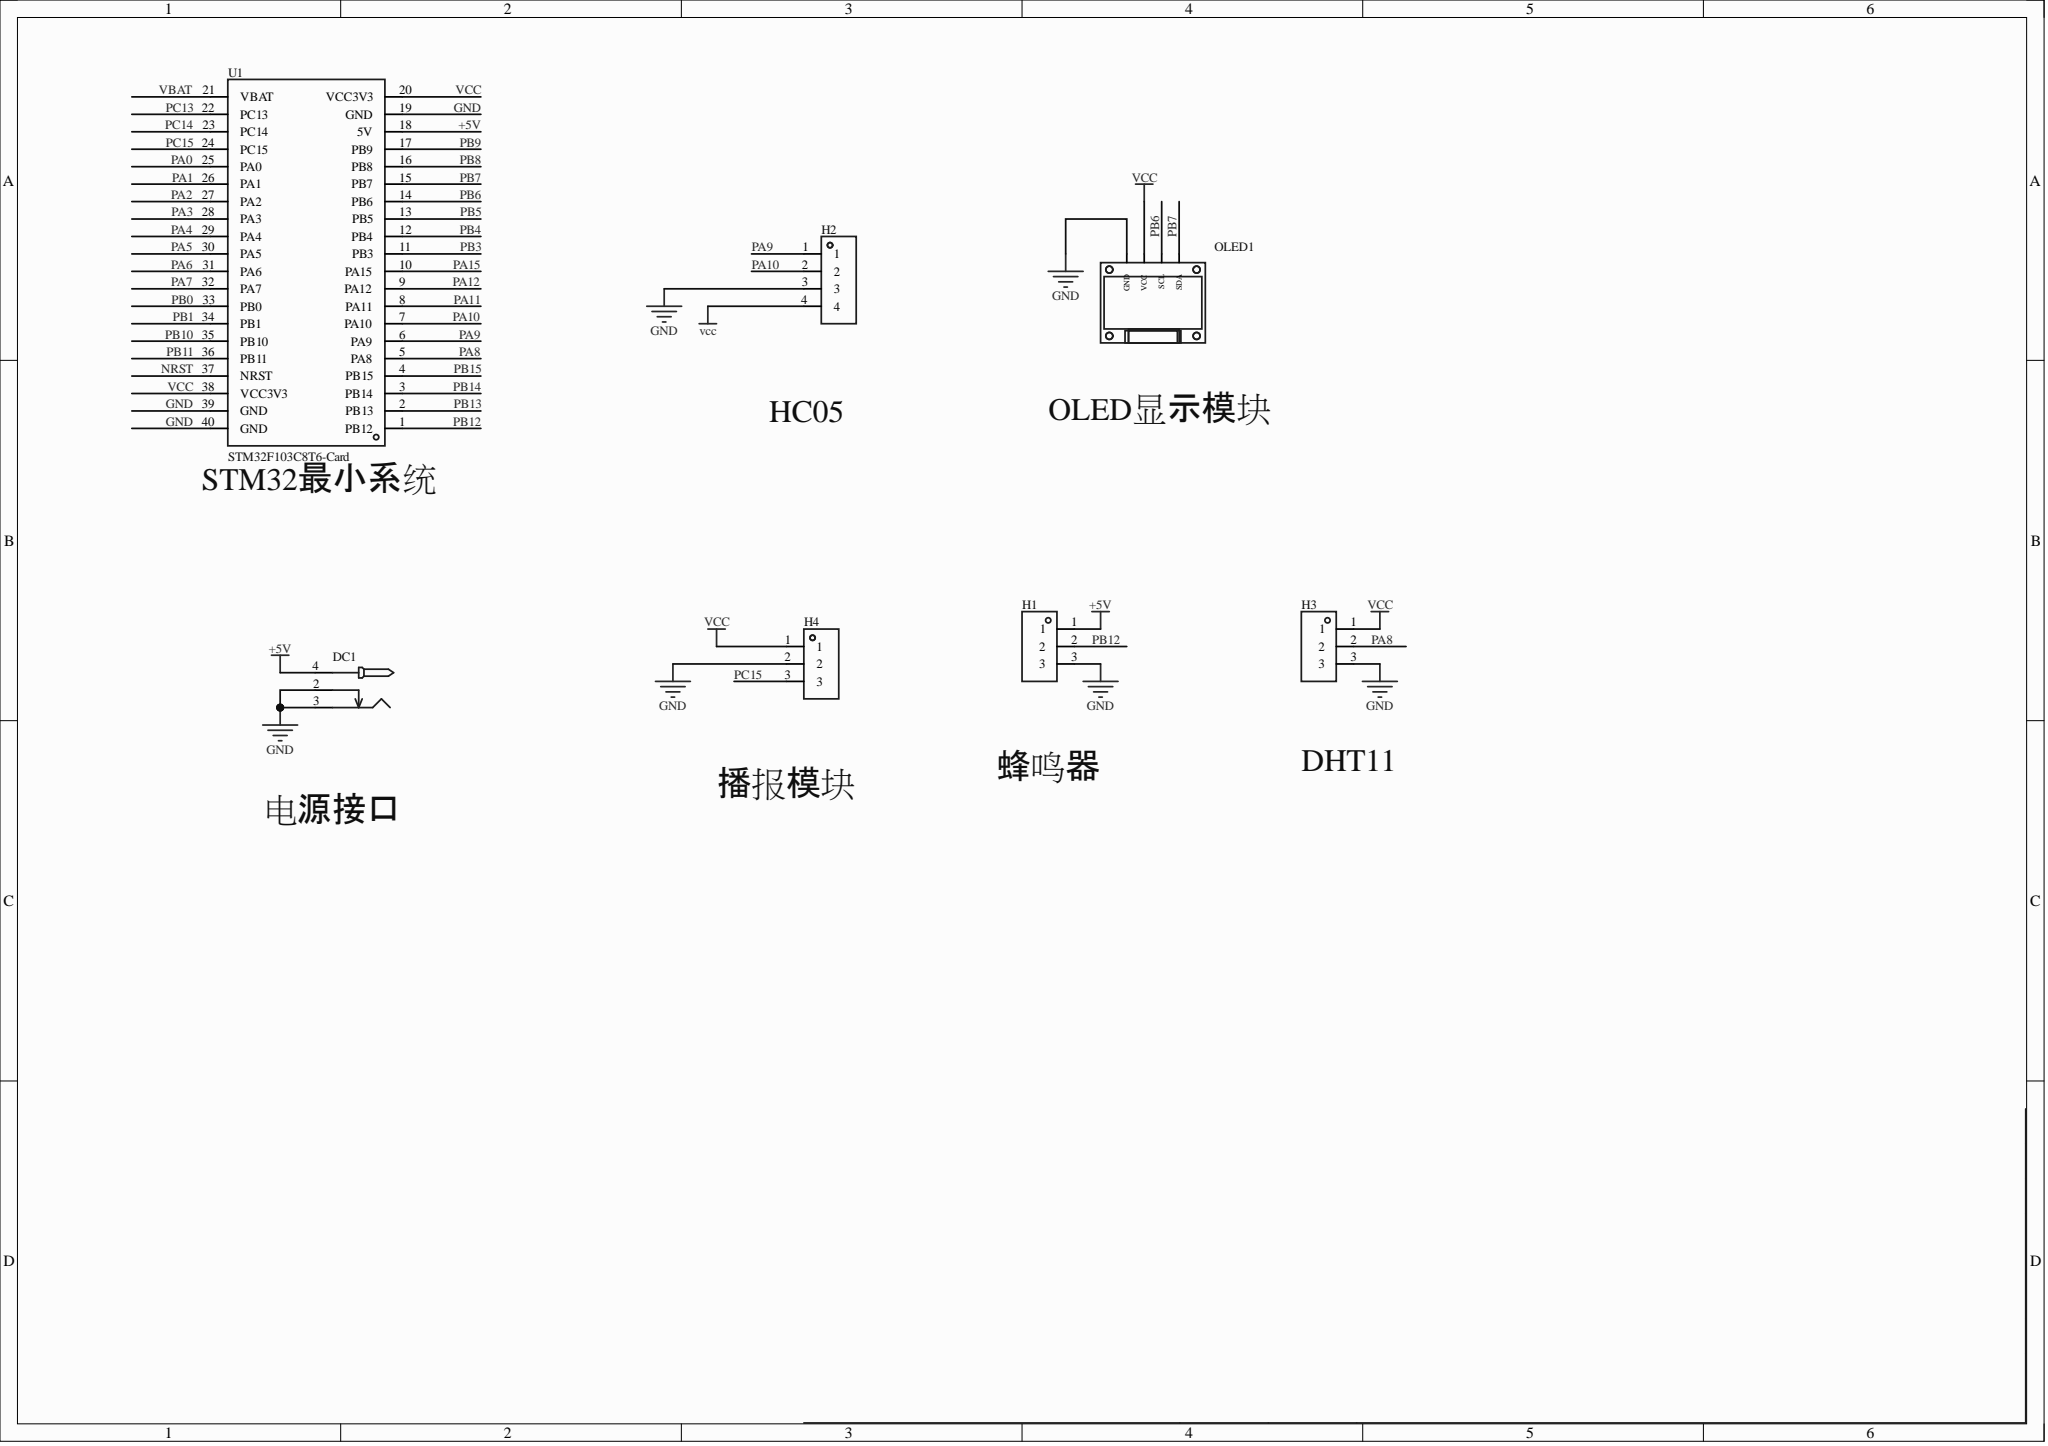Circuit board | Altium Designer | 7 parts | 10 nets
Bill of materials:
Comment,Description,Designator,Footprint,LibRef,Quantity
"","","DC1","DC-2.0","DC-005_2.0","1"
"","","H1, H3","HDR-TH_3P-P2.54-V-F","HDR-F_2.54_1x3P","2"
"","","H2","HDR-TH_4P-P2.54-V-F","HDR-F_2.54_1x4P","1"
"","","H4","HDR-TH_3P-P2.54-V-M","HDR-M_2.54_1x3P","1"
"","","OLED1","0.96OLED_4P","0.96OLED模块_4P","1"
"STM32F103C8T6-Card","","U1","CONN-TH_L53.3-W22.9_STM32F103C8T6-CARD","STM32F103C8T6-Card","1"
Netlist (Protel format):
[
DC1
DC-2.0




]
[
H1
HDR-TH_3P-P2.54-V-F




]
[
H2
HDR-TH_4P-P2.54-V-F




]
[
H3
HDR-TH_3P-P2.54-V-F




]
[
H4
HDR-TH_3P-P2.54-V-M




]
[
OLED1
0.96OLED_4P




]
[
U1
CONN-TH_L53.3-W22.9_STM32F103C8T6-CARD
STM32F103C8T6-Card



]
(
VCC
H2-4
H3-1
H4-1
OLED1-2
U1-20
U1-38
)
(
PC15
H4-3
U1-24
)
(
PB12
H1-2
U1-1
)
(
PB7
OLED1-4
U1-15
)
(
PB6
OLED1-3
U1-14
)
(
PA10
H2-2
U1-7
)
(
PA9
H2-1
U1-6
)
(
PA8
H3-2
U1-5
)
(
GND
DC1-2
DC1-3
H1-3
H2-3
H3-3
H4-2
OLED1-1
U1-19
U1-39
U1-40
)
(
+5V
DC1-4
H1-1
U1-18
)